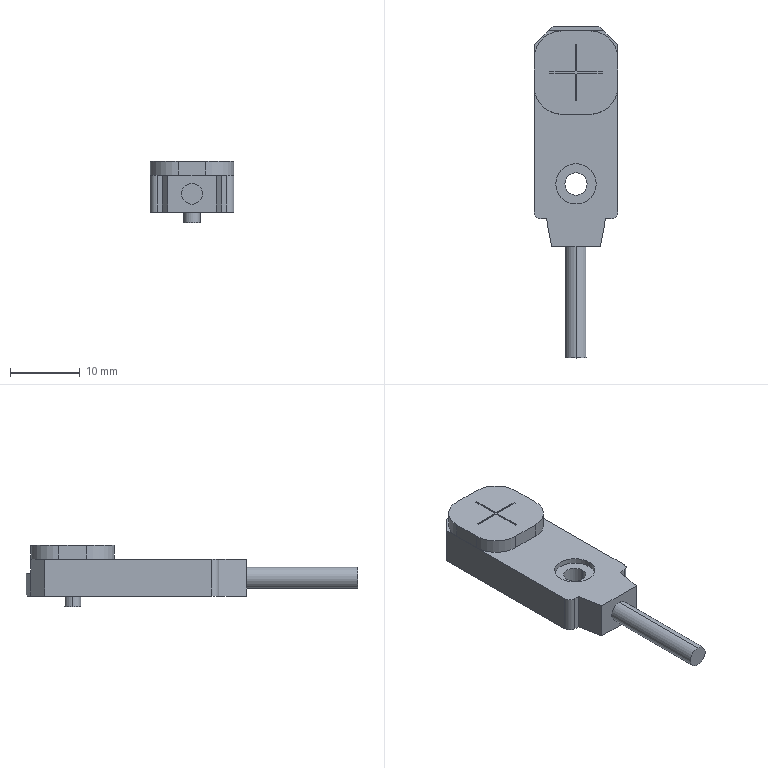Part | STEP file | square proximity sensor GX-F12A | 2 solids | 60 faces | box 12 x 47.7 x 8.8 mm | volume 2173 mm3 | plane 42 | cylinder 18 | commonest cylinder face diameters 0.5 x4 8 x4 2 x2 2.3 x2 3 x2 3.2 x2